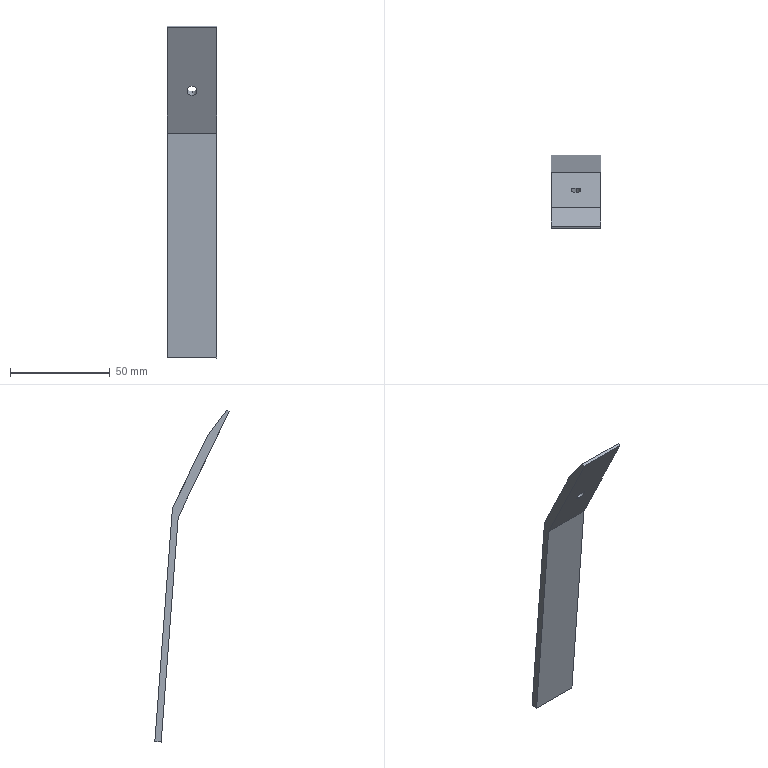Part | SolidWorks | features BaseBody 1 | 1 solid | 11 faces | box 25 x 37.198 x 166.136 mm | volume 14976 mm3 | plane 9 | cylinder 2 | commonest cylinder face diameters 5 x2
STEP:
#1=CARTESIAN_POINT('',(0.,21.96,2174.949));
#2=VERTEX_POINT('',#1);
#3=CARTESIAN_POINT('',(0.,24.129,2170.444));
#4=VERTEX_POINT('',#3);
#5=CARTESIAN_POINT('',(0.,23.045,2172.696));
#6=DIRECTION('',(0.,-0.901,-0.4339));
#7=DIRECTION('',(0.,-0.4339,0.901));
#8=AXIS2_PLACEMENT_3D('',#5,#6,#7);
#9=CIRCLE('',#8,2.5);
#10=EDGE_CURVE('',#2,#4,#9,.T.);
#11=ORIENTED_EDGE('',*,*,#10,.T.);
#12=CARTESIAN_POINT('',(0.,28.184,2172.397));
#13=VERTEX_POINT('',#12);
#14=CARTESIAN_POINT('',(0.,24.129,2170.444));
#15=DIRECTION('',(0.,0.901,0.4339));
#16=VECTOR('',#15,1000.);
#17=LINE('',#14,#16);
#18=EDGE_CURVE('',#4,#13,#17,.T.);
#19=ORIENTED_EDGE('',*,*,#18,.T.);
#20=CARTESIAN_POINT('',(0.,26.014,2176.901));
#21=VERTEX_POINT('',#20);
#22=CARTESIAN_POINT('',(0.,27.099,2174.649));
#23=DIRECTION('',(0.,0.901,0.4339));
#24=DIRECTION('',(0.,-0.4339,0.901));
#25=AXIS2_PLACEMENT_3D('',#22,#23,#24);
#26=CIRCLE('',#25,2.5);
#27=EDGE_CURVE('',#13,#21,#26,.T.);
#28=ORIENTED_EDGE('',*,*,#27,.T.);
#29=CARTESIAN_POINT('',(0.,21.96,2174.949));
#30=DIRECTION('',(0.,0.901,0.4339));
#31=VECTOR('',#30,1000.);
#32=LINE('',#29,#31);
#33=EDGE_CURVE('',#2,#21,#32,.T.);
#34=ORIENTED_EDGE('',*,*,#33,.F.);
#35=EDGE_LOOP('',(#11,#19,#28,#34));
#36=FACE_OUTER_BOUND('',#35,.T.);
#37=CARTESIAN_POINT('',(0.,23.045,2172.696));
#38=DIRECTION('',(0.,0.901,0.4339));
#39=DIRECTION('',(0.,-0.4339,0.901));
#40=AXIS2_PLACEMENT_3D('',#37,#38,#39);
#41=CYLINDRICAL_SURFACE('',#40,2.5);
#42=ADVANCED_FACE('',(#36),#41,.F.);
#43=ORIENTED_EDGE('',*,*,#18,.F.);
#44=CARTESIAN_POINT('',(0.,23.045,2172.696));
#45=DIRECTION('',(0.,-0.901,-0.4339));
#46=DIRECTION('',(0.,-0.4339,0.901));
#47=AXIS2_PLACEMENT_3D('',#44,#45,#46);
#48=CIRCLE('',#47,2.5);
#49=EDGE_CURVE('',#4,#2,#48,.T.);
#50=ORIENTED_EDGE('',*,*,#49,.T.);
#51=ORIENTED_EDGE('',*,*,#33,.T.);
#52=CARTESIAN_POINT('',(0.,27.099,2174.649));
#53=DIRECTION('',(0.,0.901,0.4339));
#54=DIRECTION('',(0.,-0.4339,0.901));
#55=AXIS2_PLACEMENT_3D('',#52,#53,#54);
#56=CIRCLE('',#55,2.5);
#57=EDGE_CURVE('',#21,#13,#56,.T.);
#58=ORIENTED_EDGE('',*,*,#57,.T.);
#59=EDGE_LOOP('',(#43,#50,#51,#58));
#60=FACE_OUTER_BOUND('',#59,.T.);
#61=CARTESIAN_POINT('',(0.,23.045,2172.696));
#62=DIRECTION('',(0.,0.901,0.4339));
#63=DIRECTION('',(0.,-0.4339,0.901));
#64=AXIS2_PLACEMENT_3D('',#61,#62,#63);
#65=CYLINDRICAL_SURFACE('',#64,2.5);
#66=ADVANCED_FACE('',(#60),#65,.F.);
#67=ORIENTED_EDGE('',*,*,#57,.F.);
#68=ORIENTED_EDGE('',*,*,#27,.F.);
#69=EDGE_LOOP('',(#67,#68));
#70=FACE_BOUND('',#69,.T.);
#71=CARTESIAN_POINT('',(12.5,18.515,2192.474));
#72=VERTEX_POINT('',#71);
#73=CARTESIAN_POINT('',(-12.5,18.515,2192.474));
#74=VERTEX_POINT('',#73);
#75=CARTESIAN_POINT('',(0.,18.515,2192.474));
#76=DIRECTION('',(-1.,0.,0.));
#77=VECTOR('',#76,1000.);
#78=LINE('',#75,#77);
#79=EDGE_CURVE('',#72,#74,#78,.T.);
#80=ORIENTED_EDGE('',*,*,#79,.F.);
#81=CARTESIAN_POINT('',(12.5,36.102,2155.955));
#82=VERTEX_POINT('',#81);
#83=CARTESIAN_POINT('',(12.5,27.308,2174.214));
#84=DIRECTION('',(0.,-0.4339,0.901));
#85=VECTOR('',#84,1000.);
#86=LINE('',#83,#85);
#87=EDGE_CURVE('',#82,#72,#86,.T.);
#88=ORIENTED_EDGE('',*,*,#87,.F.);
#89=CARTESIAN_POINT('',(-12.5,36.102,2155.955));
#90=VERTEX_POINT('',#89);
#91=CARTESIAN_POINT('',(0.,36.102,2155.955));
#92=DIRECTION('',(1.,0.,0.));
#93=VECTOR('',#92,1000.);
#94=LINE('',#91,#93);
#95=EDGE_CURVE('',#90,#82,#94,.T.);
#96=ORIENTED_EDGE('',*,*,#95,.F.);
#97=CARTESIAN_POINT('',(-12.5,27.308,2174.214));
#98=DIRECTION('',(0.,0.4339,-0.901));
#99=VECTOR('',#98,1000.);
#100=LINE('',#97,#99);
#101=EDGE_CURVE('',#74,#90,#100,.T.);
#102=ORIENTED_EDGE('',*,*,#101,.F.);
#103=EDGE_LOOP('',(#80,#88,#96,#102));
#104=FACE_OUTER_BOUND('',#103,.T.);
#105=CARTESIAN_POINT('',(-12.5,18.515,2192.474));
#106=DIRECTION('',(0.,-0.901,-0.4339));
#107=DIRECTION('',(0.,0.4339,-0.901));
#108=AXIS2_PLACEMENT_3D('',#105,#106,#107);
#109=PLANE('',#108);
#110=ADVANCED_FACE('',(#70,#104),#109,.F.);
#111=ORIENTED_EDGE('',*,*,#10,.F.);
#112=ORIENTED_EDGE('',*,*,#49,.F.);
#113=EDGE_LOOP('',(#111,#112));
#114=FACE_BOUND('',#113,.T.);
#115=CARTESIAN_POINT('',(12.5,33.224,2151.559));
#116=VERTEX_POINT('',#115);
#117=CARTESIAN_POINT('',(-12.5,33.224,2151.559));
#118=VERTEX_POINT('',#117);
#119=CARTESIAN_POINT('',(0.,33.224,2151.559));
#120=DIRECTION('',(-1.,0.,0.));
#121=VECTOR('',#120,1000.);
#122=LINE('',#119,#121);
#123=EDGE_CURVE('',#116,#118,#122,.T.);
#124=ORIENTED_EDGE('',*,*,#123,.F.);
#125=CARTESIAN_POINT('',(12.5,7.699,2204.561));
#126=VERTEX_POINT('',#125);
#127=CARTESIAN_POINT('',(12.5,20.462,2178.06));
#128=DIRECTION('',(0.,0.4339,-0.901));
#129=VECTOR('',#128,1000.);
#130=LINE('',#127,#129);
#131=EDGE_CURVE('',#126,#116,#130,.T.);
#132=ORIENTED_EDGE('',*,*,#131,.F.);
#133=CARTESIAN_POINT('',(-12.5,7.699,2204.561));
#134=VERTEX_POINT('',#133);
#135=CARTESIAN_POINT('',(0.,7.699,2204.561));
#136=DIRECTION('',(1.,0.,0.));
#137=VECTOR('',#136,1000.);
#138=LINE('',#135,#137);
#139=EDGE_CURVE('',#134,#126,#138,.T.);
#140=ORIENTED_EDGE('',*,*,#139,.F.);
#141=CARTESIAN_POINT('',(-12.5,20.462,2178.06));
#142=DIRECTION('',(0.,-0.4339,0.901));
#143=VECTOR('',#142,1000.);
#144=LINE('',#141,#143);
#145=EDGE_CURVE('',#118,#134,#144,.T.);
#146=ORIENTED_EDGE('',*,*,#145,.F.);
#147=EDGE_LOOP('',(#124,#132,#140,#146));
#148=FACE_OUTER_BOUND('',#147,.T.);
#149=CARTESIAN_POINT('',(-12.5,33.224,2151.559));
#150=DIRECTION('',(0.,0.901,0.4339));
#151=DIRECTION('',(0.,-0.4339,0.901));
#152=AXIS2_PLACEMENT_3D('',#149,#150,#151);
#153=PLANE('',#152);
#154=ADVANCED_FACE('',(#114,#148),#153,.F.);
#155=CARTESIAN_POINT('',(-12.5,9.012,2205.181));
#156=VERTEX_POINT('',#155);
#157=CARTESIAN_POINT('',(-12.5,9.012,2205.181));
#158=DIRECTION('',(0.,0.5989,-0.8008));
#159=VECTOR('',#158,1000.);
#160=LINE('',#157,#159);
#161=EDGE_CURVE('',#156,#74,#160,.T.);
#162=ORIENTED_EDGE('',*,*,#161,.T.);
#163=ORIENTED_EDGE('',*,*,#101,.T.);
#164=CARTESIAN_POINT('',(-12.5,44.897,2039.286));
#165=VERTEX_POINT('',#164);
#166=CARTESIAN_POINT('',(-12.5,36.102,2155.955));
#167=DIRECTION('',(0.,0.07517,-0.9972));
#168=VECTOR('',#167,1000.);
#169=LINE('',#166,#168);
#170=EDGE_CURVE('',#90,#165,#169,.T.);
#171=ORIENTED_EDGE('',*,*,#170,.T.);
#172=CARTESIAN_POINT('',(-12.5,41.706,2039.046));
#173=VERTEX_POINT('',#172);
#174=CARTESIAN_POINT('',(-12.5,44.897,2039.286));
#175=DIRECTION('',(0.,-0.9972,-0.07517));
#176=VECTOR('',#175,1000.);
#177=LINE('',#174,#176);
#178=EDGE_CURVE('',#165,#173,#177,.T.);
#179=ORIENTED_EDGE('',*,*,#178,.T.);
#180=CARTESIAN_POINT('',(-12.5,41.706,2039.046));
#181=DIRECTION('',(0.,-0.07517,0.9972));
#182=VECTOR('',#181,1000.);
#183=LINE('',#180,#182);
#184=EDGE_CURVE('',#173,#118,#183,.T.);
#185=ORIENTED_EDGE('',*,*,#184,.T.);
#186=ORIENTED_EDGE('',*,*,#145,.T.);
#187=CARTESIAN_POINT('',(-12.5,7.699,2204.561));
#188=DIRECTION('',(0.,0.904,0.4275));
#189=VECTOR('',#188,1000.);
#190=LINE('',#187,#189);
#191=EDGE_CURVE('',#134,#156,#190,.T.);
#192=ORIENTED_EDGE('',*,*,#191,.T.);
#193=EDGE_LOOP('',(#162,#163,#171,#179,#185,#186,#192));
#194=FACE_OUTER_BOUND('',#193,.T.);
#195=CARTESIAN_POINT('',(-12.5,7.699,2039.046));
#196=DIRECTION('',(-1.,0.,0.));
#197=DIRECTION('',(0.,0.,1.));
#198=AXIS2_PLACEMENT_3D('',#195,#196,#197);
#199=PLANE('',#198);
#200=ADVANCED_FACE('',(#194),#199,.T.);
#201=CARTESIAN_POINT('',(12.5,9.012,2205.181));
#202=VERTEX_POINT('',#201);
#203=CARTESIAN_POINT('',(0.,9.012,2205.181));
#204=DIRECTION('',(-1.,0.,0.));
#205=VECTOR('',#204,1000.);
#206=LINE('',#203,#205);
#207=EDGE_CURVE('',#202,#156,#206,.T.);
#208=ORIENTED_EDGE('',*,*,#207,.F.);
#209=CARTESIAN_POINT('',(12.5,13.763,2198.828));
#210=DIRECTION('',(0.,-0.5989,0.8008));
#211=VECTOR('',#210,1000.);
#212=LINE('',#209,#211);
#213=EDGE_CURVE('',#72,#202,#212,.T.);
#214=ORIENTED_EDGE('',*,*,#213,.F.);
#215=ORIENTED_EDGE('',*,*,#79,.T.);
#216=ORIENTED_EDGE('',*,*,#161,.F.);
#217=EDGE_LOOP('',(#208,#214,#215,#216));
#218=FACE_OUTER_BOUND('',#217,.T.);
#219=CARTESIAN_POINT('',(-12.5,9.012,2205.181));
#220=DIRECTION('',(0.,-0.8008,-0.5989));
#221=DIRECTION('',(0.,0.5989,-0.8008));
#222=AXIS2_PLACEMENT_3D('',#219,#220,#221);
#223=PLANE('',#222);
#224=ADVANCED_FACE('',(#218),#223,.F.);
#225=ORIENTED_EDGE('',*,*,#87,.T.);
#226=ORIENTED_EDGE('',*,*,#213,.T.);
#227=CARTESIAN_POINT('',(12.5,7.699,2204.561));
#228=DIRECTION('',(0.,0.904,0.4275));
#229=VECTOR('',#228,1000.);
#230=LINE('',#227,#229);
#231=EDGE_CURVE('',#126,#202,#230,.T.);
#232=ORIENTED_EDGE('',*,*,#231,.F.);
#233=ORIENTED_EDGE('',*,*,#131,.T.);
#234=CARTESIAN_POINT('',(12.5,41.706,2039.046));
#235=VERTEX_POINT('',#234);
#236=CARTESIAN_POINT('',(12.5,41.706,2039.046));
#237=DIRECTION('',(0.,-0.07517,0.9972));
#238=VECTOR('',#237,1000.);
#239=LINE('',#236,#238);
#240=EDGE_CURVE('',#235,#116,#239,.T.);
#241=ORIENTED_EDGE('',*,*,#240,.F.);
#242=CARTESIAN_POINT('',(12.5,44.897,2039.286));
#243=VERTEX_POINT('',#242);
#244=CARTESIAN_POINT('',(12.5,44.897,2039.286));
#245=DIRECTION('',(0.,-0.9972,-0.07517));
#246=VECTOR('',#245,1000.);
#247=LINE('',#244,#246);
#248=EDGE_CURVE('',#243,#235,#247,.T.);
#249=ORIENTED_EDGE('',*,*,#248,.F.);
#250=CARTESIAN_POINT('',(12.5,36.102,2155.955));
#251=DIRECTION('',(0.,0.07517,-0.9972));
#252=VECTOR('',#251,1000.);
#253=LINE('',#250,#252);
#254=EDGE_CURVE('',#82,#243,#253,.T.);
#255=ORIENTED_EDGE('',*,*,#254,.F.);
#256=EDGE_LOOP('',(#225,#226,#232,#233,#241,#249,#255));
#257=FACE_OUTER_BOUND('',#256,.T.);
#258=CARTESIAN_POINT('',(12.5,7.699,2039.046));
#259=DIRECTION('',(-1.,0.,0.));
#260=DIRECTION('',(0.,0.,1.));
#261=AXIS2_PLACEMENT_3D('',#258,#259,#260);
#262=PLANE('',#261);
#263=ADVANCED_FACE('',(#257),#262,.F.);
#264=ORIENTED_EDGE('',*,*,#95,.T.);
#265=ORIENTED_EDGE('',*,*,#254,.T.);
#266=CARTESIAN_POINT('',(0.,44.897,2039.286));
#267=DIRECTION('',(1.,0.,0.));
#268=VECTOR('',#267,1000.);
#269=LINE('',#266,#268);
#270=EDGE_CURVE('',#165,#243,#269,.T.);
#271=ORIENTED_EDGE('',*,*,#270,.F.);
#272=ORIENTED_EDGE('',*,*,#170,.F.);
#273=EDGE_LOOP('',(#264,#265,#271,#272));
#274=FACE_OUTER_BOUND('',#273,.T.);
#275=CARTESIAN_POINT('',(-12.5,36.102,2155.955));
#276=DIRECTION('',(0.,-0.9972,-0.07517));
#277=DIRECTION('',(0.,0.07517,-0.9972));
#278=AXIS2_PLACEMENT_3D('',#275,#276,#277);
#279=PLANE('',#278);
#280=ADVANCED_FACE('',(#274),#279,.F.);
#281=CARTESIAN_POINT('',(0.,41.706,2039.046));
#282=DIRECTION('',(-1.,0.,0.));
#283=VECTOR('',#282,1000.);
#284=LINE('',#281,#283);
#285=EDGE_CURVE('',#235,#173,#284,.T.);
#286=ORIENTED_EDGE('',*,*,#285,.F.);
#287=ORIENTED_EDGE('',*,*,#240,.T.);
#288=ORIENTED_EDGE('',*,*,#123,.T.);
#289=ORIENTED_EDGE('',*,*,#184,.F.);
#290=EDGE_LOOP('',(#286,#287,#288,#289));
#291=FACE_OUTER_BOUND('',#290,.T.);
#292=CARTESIAN_POINT('',(-12.5,41.706,2039.046));
#293=DIRECTION('',(0.,0.9972,0.07517));
#294=DIRECTION('',(0.,-0.07517,0.9972));
#295=AXIS2_PLACEMENT_3D('',#292,#293,#294);
#296=PLANE('',#295);
#297=ADVANCED_FACE('',(#291),#296,.F.);
#298=ORIENTED_EDGE('',*,*,#139,.T.);
#299=ORIENTED_EDGE('',*,*,#231,.T.);
#300=ORIENTED_EDGE('',*,*,#207,.T.);
#301=ORIENTED_EDGE('',*,*,#191,.F.);
#302=EDGE_LOOP('',(#298,#299,#300,#301));
#303=FACE_OUTER_BOUND('',#302,.T.);
#304=CARTESIAN_POINT('',(-12.5,7.699,2204.561));
#305=DIRECTION('',(0.,0.4275,-0.904));
#306=DIRECTION('',(0.,0.904,0.4275));
#307=AXIS2_PLACEMENT_3D('',#304,#305,#306);
#308=PLANE('',#307);
#309=ADVANCED_FACE('',(#303),#308,.F.);
#310=ORIENTED_EDGE('',*,*,#270,.T.);
#311=ORIENTED_EDGE('',*,*,#248,.T.);
#312=ORIENTED_EDGE('',*,*,#285,.T.);
#313=ORIENTED_EDGE('',*,*,#178,.F.);
#314=EDGE_LOOP('',(#310,#311,#312,#313));
#315=FACE_OUTER_BOUND('',#314,.T.);
#316=CARTESIAN_POINT('',(-12.5,44.897,2039.286));
#317=DIRECTION('',(0.,-0.07517,0.9972));
#318=DIRECTION('',(0.,-0.9972,-0.07517));
#319=AXIS2_PLACEMENT_3D('',#316,#317,#318);
#320=PLANE('',#319);
#321=ADVANCED_FACE('',(#315),#320,.F.);
#322=CLOSED_SHELL('',(#42,#66,#110,#154,#200,#224,#263,#280,#297,#309,#321));
#323=MANIFOLD_SOLID_BREP('',#322);
#324=CARTESIAN_POINT('',(0.,0.,0.));
#325=DIRECTION('',(0.,0.,1.));
#326=DIRECTION('',(1.,0.,0.));
#327=AXIS2_PLACEMENT_3D('',#324,#325,#326);
#328=(LENGTH_UNIT()NAMED_UNIT(*)SI_UNIT(.MILLI.,.METRE.));
#329=UNCERTAINTY_MEASURE_WITH_UNIT(LENGTH_MEASURE(0.00001),#328,'','');
#330=(NAMED_UNIT(*)PLANE_ANGLE_UNIT()SI_UNIT($,.RADIAN.));
#331=(NAMED_UNIT(*)SI_UNIT($,.STERADIAN.)SOLID_ANGLE_UNIT());
#332=(GEOMETRIC_REPRESENTATION_CONTEXT(3)GLOBAL_UNCERTAINTY_ASSIGNED_CONTEXT((#329))GLOBAL_UNIT_ASSIGNED_CONTEXT((#328,#330,#331))REPRESENTATION_CONTEXT('',''));
#333=ADVANCED_BREP_SHAPE_REPRESENTATION('',(#323,#327),#332);